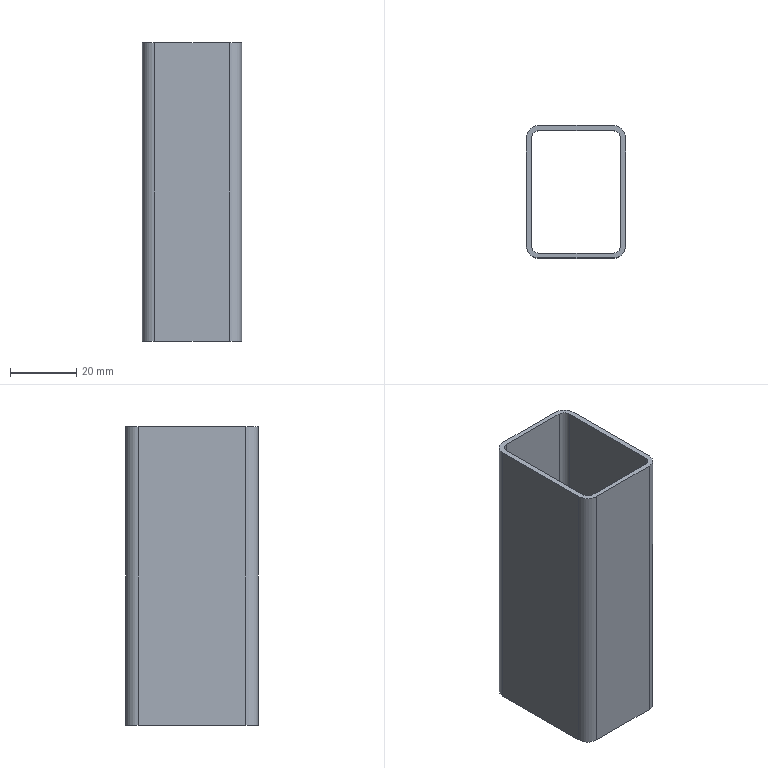Part | SolidWorks | features BaseBody 1 | 1 solid | 18 faces | box 30 x 40 x 90 mm | volume 17395 mm3 | plane 10 | cylinder 8 | commonest cylinder face diameters 4.5 x4 7.5 x4
STEP:
#1=CARTESIAN_POINT('',(11.25,18.5,90.));
#2=VERTEX_POINT('',#1);
#3=CARTESIAN_POINT('',(-11.25,18.5,90.));
#4=VERTEX_POINT('',#3);
#5=CARTESIAN_POINT('',(-5.625,18.5,90.));
#6=DIRECTION('',(-1.,0.,0.));
#7=VECTOR('',#6,1000.);
#8=LINE('',#5,#7);
#9=EDGE_CURVE('',#2,#4,#8,.T.);
#10=ORIENTED_EDGE('',*,*,#9,.F.);
#11=CARTESIAN_POINT('',(13.5,16.25,90.));
#12=VERTEX_POINT('',#11);
#13=CARTESIAN_POINT('',(11.25,16.25,90.));
#14=DIRECTION('',(0.,0.,1.));
#15=DIRECTION('',(-1.,0.,0.));
#16=AXIS2_PLACEMENT_3D('',#13,#14,#15);
#17=CIRCLE('',#16,2.25);
#18=EDGE_CURVE('',#12,#2,#17,.T.);
#19=ORIENTED_EDGE('',*,*,#18,.F.);
#20=CARTESIAN_POINT('',(13.5,-16.25,90.));
#21=VERTEX_POINT('',#20);
#22=CARTESIAN_POINT('',(13.5,8.125,90.));
#23=DIRECTION('',(0.,1.,0.));
#24=VECTOR('',#23,1000.);
#25=LINE('',#22,#24);
#26=EDGE_CURVE('',#21,#12,#25,.T.);
#27=ORIENTED_EDGE('',*,*,#26,.F.);
#28=CARTESIAN_POINT('',(11.25,-18.5,90.));
#29=VERTEX_POINT('',#28);
#30=CARTESIAN_POINT('',(11.25,-16.25,90.));
#31=DIRECTION('',(0.,0.,1.));
#32=DIRECTION('',(0.,1.,0.));
#33=AXIS2_PLACEMENT_3D('',#30,#31,#32);
#34=CIRCLE('',#33,2.25);
#35=EDGE_CURVE('',#29,#21,#34,.T.);
#36=ORIENTED_EDGE('',*,*,#35,.F.);
#37=CARTESIAN_POINT('',(-11.25,-18.5,90.));
#38=VERTEX_POINT('',#37);
#39=CARTESIAN_POINT('',(5.625,-18.5,90.));
#40=DIRECTION('',(1.,0.,0.));
#41=VECTOR('',#40,1000.);
#42=LINE('',#39,#41);
#43=EDGE_CURVE('',#38,#29,#42,.T.);
#44=ORIENTED_EDGE('',*,*,#43,.F.);
#45=CARTESIAN_POINT('',(-13.5,-16.25,90.));
#46=VERTEX_POINT('',#45);
#47=CARTESIAN_POINT('',(-11.25,-16.25,90.));
#48=DIRECTION('',(0.,0.,1.));
#49=DIRECTION('',(1.,0.,0.));
#50=AXIS2_PLACEMENT_3D('',#47,#48,#49);
#51=CIRCLE('',#50,2.25);
#52=EDGE_CURVE('',#46,#38,#51,.T.);
#53=ORIENTED_EDGE('',*,*,#52,.F.);
#54=CARTESIAN_POINT('',(-13.5,16.25,90.));
#55=VERTEX_POINT('',#54);
#56=CARTESIAN_POINT('',(-13.5,-8.125,90.));
#57=DIRECTION('',(0.,-1.,0.));
#58=VECTOR('',#57,1000.);
#59=LINE('',#56,#58);
#60=EDGE_CURVE('',#55,#46,#59,.T.);
#61=ORIENTED_EDGE('',*,*,#60,.F.);
#62=CARTESIAN_POINT('',(-11.25,16.25,90.));
#63=DIRECTION('',(0.,0.,1.));
#64=DIRECTION('',(0.,-1.,0.));
#65=AXIS2_PLACEMENT_3D('',#62,#63,#64);
#66=CIRCLE('',#65,2.25);
#67=EDGE_CURVE('',#4,#55,#66,.T.);
#68=ORIENTED_EDGE('',*,*,#67,.F.);
#69=EDGE_LOOP('',(#10,#19,#27,#36,#44,#53,#61,#68));
#70=FACE_BOUND('',#69,.T.);
#71=CARTESIAN_POINT('',(-15.,-16.25,90.));
#72=VERTEX_POINT('',#71);
#73=CARTESIAN_POINT('',(-15.,16.25,90.));
#74=VERTEX_POINT('',#73);
#75=CARTESIAN_POINT('',(-15.,-8.125,90.));
#76=DIRECTION('',(0.,1.,0.));
#77=VECTOR('',#76,1000.);
#78=LINE('',#75,#77);
#79=EDGE_CURVE('',#72,#74,#78,.T.);
#80=ORIENTED_EDGE('',*,*,#79,.F.);
#81=CARTESIAN_POINT('',(-11.25,-20.,90.));
#82=VERTEX_POINT('',#81);
#83=CARTESIAN_POINT('',(-11.25,-16.25,90.));
#84=DIRECTION('',(0.,0.,-1.));
#85=DIRECTION('',(1.,0.,0.));
#86=AXIS2_PLACEMENT_3D('',#83,#84,#85);
#87=CIRCLE('',#86,3.75);
#88=EDGE_CURVE('',#82,#72,#87,.T.);
#89=ORIENTED_EDGE('',*,*,#88,.F.);
#90=CARTESIAN_POINT('',(11.25,-20.,90.));
#91=VERTEX_POINT('',#90);
#92=CARTESIAN_POINT('',(5.625,-20.,90.));
#93=DIRECTION('',(-1.,0.,0.));
#94=VECTOR('',#93,1000.);
#95=LINE('',#92,#94);
#96=EDGE_CURVE('',#91,#82,#95,.T.);
#97=ORIENTED_EDGE('',*,*,#96,.F.);
#98=CARTESIAN_POINT('',(15.,-16.25,90.));
#99=VERTEX_POINT('',#98);
#100=CARTESIAN_POINT('',(11.25,-16.25,90.));
#101=DIRECTION('',(0.,0.,-1.));
#102=DIRECTION('',(0.,1.,0.));
#103=AXIS2_PLACEMENT_3D('',#100,#101,#102);
#104=CIRCLE('',#103,3.75);
#105=EDGE_CURVE('',#99,#91,#104,.T.);
#106=ORIENTED_EDGE('',*,*,#105,.F.);
#107=CARTESIAN_POINT('',(15.,16.25,90.));
#108=VERTEX_POINT('',#107);
#109=CARTESIAN_POINT('',(15.,8.125,90.));
#110=DIRECTION('',(0.,-1.,0.));
#111=VECTOR('',#110,1000.);
#112=LINE('',#109,#111);
#113=EDGE_CURVE('',#108,#99,#112,.T.);
#114=ORIENTED_EDGE('',*,*,#113,.F.);
#115=CARTESIAN_POINT('',(11.25,20.,90.));
#116=VERTEX_POINT('',#115);
#117=CARTESIAN_POINT('',(11.25,16.25,90.));
#118=DIRECTION('',(0.,0.,-1.));
#119=DIRECTION('',(-1.,0.,0.));
#120=AXIS2_PLACEMENT_3D('',#117,#118,#119);
#121=CIRCLE('',#120,3.75);
#122=EDGE_CURVE('',#116,#108,#121,.T.);
#123=ORIENTED_EDGE('',*,*,#122,.F.);
#124=CARTESIAN_POINT('',(-11.25,20.,90.));
#125=VERTEX_POINT('',#124);
#126=CARTESIAN_POINT('',(-5.625,20.,90.));
#127=DIRECTION('',(1.,0.,0.));
#128=VECTOR('',#127,1000.);
#129=LINE('',#126,#128);
#130=EDGE_CURVE('',#125,#116,#129,.T.);
#131=ORIENTED_EDGE('',*,*,#130,.F.);
#132=CARTESIAN_POINT('',(-11.25,16.25,90.));
#133=DIRECTION('',(0.,0.,-1.));
#134=DIRECTION('',(0.,-1.,0.));
#135=AXIS2_PLACEMENT_3D('',#132,#133,#134);
#136=CIRCLE('',#135,3.75);
#137=EDGE_CURVE('',#74,#125,#136,.T.);
#138=ORIENTED_EDGE('',*,*,#137,.F.);
#139=EDGE_LOOP('',(#80,#89,#97,#106,#114,#123,#131,#138));
#140=FACE_OUTER_BOUND('',#139,.T.);
#141=CARTESIAN_POINT('',(0.,0.,90.));
#142=DIRECTION('',(0.,0.,1.));
#143=DIRECTION('',(1.,0.,0.));
#144=AXIS2_PLACEMENT_3D('',#141,#142,#143);
#145=PLANE('',#144);
#146=ADVANCED_FACE('',(#70,#140),#145,.T.);
#147=CARTESIAN_POINT('',(11.25,18.5,0.));
#148=VERTEX_POINT('',#147);
#149=CARTESIAN_POINT('',(-11.25,18.5,0.));
#150=VERTEX_POINT('',#149);
#151=CARTESIAN_POINT('',(-5.625,18.5,0.));
#152=DIRECTION('',(-1.,0.,0.));
#153=VECTOR('',#152,1000.);
#154=LINE('',#151,#153);
#155=EDGE_CURVE('',#148,#150,#154,.T.);
#156=ORIENTED_EDGE('',*,*,#155,.T.);
#157=CARTESIAN_POINT('',(-13.5,16.25,0.));
#158=VERTEX_POINT('',#157);
#159=CARTESIAN_POINT('',(-11.25,16.25,0.));
#160=DIRECTION('',(0.,0.,1.));
#161=DIRECTION('',(0.,-1.,0.));
#162=AXIS2_PLACEMENT_3D('',#159,#160,#161);
#163=CIRCLE('',#162,2.25);
#164=EDGE_CURVE('',#150,#158,#163,.T.);
#165=ORIENTED_EDGE('',*,*,#164,.T.);
#166=CARTESIAN_POINT('',(-13.5,-16.25,0.));
#167=VERTEX_POINT('',#166);
#168=CARTESIAN_POINT('',(-13.5,-8.125,0.));
#169=DIRECTION('',(0.,-1.,0.));
#170=VECTOR('',#169,1000.);
#171=LINE('',#168,#170);
#172=EDGE_CURVE('',#158,#167,#171,.T.);
#173=ORIENTED_EDGE('',*,*,#172,.T.);
#174=CARTESIAN_POINT('',(-11.25,-18.5,0.));
#175=VERTEX_POINT('',#174);
#176=CARTESIAN_POINT('',(-11.25,-16.25,0.));
#177=DIRECTION('',(0.,0.,1.));
#178=DIRECTION('',(1.,0.,0.));
#179=AXIS2_PLACEMENT_3D('',#176,#177,#178);
#180=CIRCLE('',#179,2.25);
#181=EDGE_CURVE('',#167,#175,#180,.T.);
#182=ORIENTED_EDGE('',*,*,#181,.T.);
#183=CARTESIAN_POINT('',(11.25,-18.5,0.));
#184=VERTEX_POINT('',#183);
#185=CARTESIAN_POINT('',(5.625,-18.5,0.));
#186=DIRECTION('',(1.,0.,0.));
#187=VECTOR('',#186,1000.);
#188=LINE('',#185,#187);
#189=EDGE_CURVE('',#175,#184,#188,.T.);
#190=ORIENTED_EDGE('',*,*,#189,.T.);
#191=CARTESIAN_POINT('',(13.5,-16.25,0.));
#192=VERTEX_POINT('',#191);
#193=CARTESIAN_POINT('',(11.25,-16.25,0.));
#194=DIRECTION('',(0.,0.,1.));
#195=DIRECTION('',(0.,1.,0.));
#196=AXIS2_PLACEMENT_3D('',#193,#194,#195);
#197=CIRCLE('',#196,2.25);
#198=EDGE_CURVE('',#184,#192,#197,.T.);
#199=ORIENTED_EDGE('',*,*,#198,.T.);
#200=CARTESIAN_POINT('',(13.5,16.25,0.));
#201=VERTEX_POINT('',#200);
#202=CARTESIAN_POINT('',(13.5,8.125,0.));
#203=DIRECTION('',(0.,1.,0.));
#204=VECTOR('',#203,1000.);
#205=LINE('',#202,#204);
#206=EDGE_CURVE('',#192,#201,#205,.T.);
#207=ORIENTED_EDGE('',*,*,#206,.T.);
#208=CARTESIAN_POINT('',(11.25,16.25,0.));
#209=DIRECTION('',(0.,0.,1.));
#210=DIRECTION('',(-1.,0.,0.));
#211=AXIS2_PLACEMENT_3D('',#208,#209,#210);
#212=CIRCLE('',#211,2.25);
#213=EDGE_CURVE('',#201,#148,#212,.T.);
#214=ORIENTED_EDGE('',*,*,#213,.T.);
#215=EDGE_LOOP('',(#156,#165,#173,#182,#190,#199,#207,#214));
#216=FACE_BOUND('',#215,.T.);
#217=CARTESIAN_POINT('',(-15.,-16.25,0.));
#218=VERTEX_POINT('',#217);
#219=CARTESIAN_POINT('',(-15.,16.25,0.));
#220=VERTEX_POINT('',#219);
#221=CARTESIAN_POINT('',(-15.,-8.125,0.));
#222=DIRECTION('',(0.,1.,0.));
#223=VECTOR('',#222,1000.);
#224=LINE('',#221,#223);
#225=EDGE_CURVE('',#218,#220,#224,.T.);
#226=ORIENTED_EDGE('',*,*,#225,.T.);
#227=CARTESIAN_POINT('',(-11.25,20.,0.));
#228=VERTEX_POINT('',#227);
#229=CARTESIAN_POINT('',(-11.25,16.25,0.));
#230=DIRECTION('',(0.,0.,-1.));
#231=DIRECTION('',(0.,-1.,0.));
#232=AXIS2_PLACEMENT_3D('',#229,#230,#231);
#233=CIRCLE('',#232,3.75);
#234=EDGE_CURVE('',#220,#228,#233,.T.);
#235=ORIENTED_EDGE('',*,*,#234,.T.);
#236=CARTESIAN_POINT('',(11.25,20.,0.));
#237=VERTEX_POINT('',#236);
#238=CARTESIAN_POINT('',(-5.625,20.,0.));
#239=DIRECTION('',(1.,0.,0.));
#240=VECTOR('',#239,1000.);
#241=LINE('',#238,#240);
#242=EDGE_CURVE('',#228,#237,#241,.T.);
#243=ORIENTED_EDGE('',*,*,#242,.T.);
#244=CARTESIAN_POINT('',(15.,16.25,0.));
#245=VERTEX_POINT('',#244);
#246=CARTESIAN_POINT('',(11.25,16.25,0.));
#247=DIRECTION('',(0.,0.,-1.));
#248=DIRECTION('',(-1.,0.,0.));
#249=AXIS2_PLACEMENT_3D('',#246,#247,#248);
#250=CIRCLE('',#249,3.75);
#251=EDGE_CURVE('',#237,#245,#250,.T.);
#252=ORIENTED_EDGE('',*,*,#251,.T.);
#253=CARTESIAN_POINT('',(15.,-16.25,0.));
#254=VERTEX_POINT('',#253);
#255=CARTESIAN_POINT('',(15.,8.125,0.));
#256=DIRECTION('',(0.,-1.,0.));
#257=VECTOR('',#256,1000.);
#258=LINE('',#255,#257);
#259=EDGE_CURVE('',#245,#254,#258,.T.);
#260=ORIENTED_EDGE('',*,*,#259,.T.);
#261=CARTESIAN_POINT('',(11.25,-20.,0.));
#262=VERTEX_POINT('',#261);
#263=CARTESIAN_POINT('',(11.25,-16.25,0.));
#264=DIRECTION('',(0.,0.,-1.));
#265=DIRECTION('',(0.,1.,0.));
#266=AXIS2_PLACEMENT_3D('',#263,#264,#265);
#267=CIRCLE('',#266,3.75);
#268=EDGE_CURVE('',#254,#262,#267,.T.);
#269=ORIENTED_EDGE('',*,*,#268,.T.);
#270=CARTESIAN_POINT('',(-11.25,-20.,0.));
#271=VERTEX_POINT('',#270);
#272=CARTESIAN_POINT('',(5.625,-20.,0.));
#273=DIRECTION('',(-1.,0.,0.));
#274=VECTOR('',#273,1000.);
#275=LINE('',#272,#274);
#276=EDGE_CURVE('',#262,#271,#275,.T.);
#277=ORIENTED_EDGE('',*,*,#276,.T.);
#278=CARTESIAN_POINT('',(-11.25,-16.25,0.));
#279=DIRECTION('',(0.,0.,-1.));
#280=DIRECTION('',(1.,0.,0.));
#281=AXIS2_PLACEMENT_3D('',#278,#279,#280);
#282=CIRCLE('',#281,3.75);
#283=EDGE_CURVE('',#271,#218,#282,.T.);
#284=ORIENTED_EDGE('',*,*,#283,.T.);
#285=EDGE_LOOP('',(#226,#235,#243,#252,#260,#269,#277,#284));
#286=FACE_OUTER_BOUND('',#285,.T.);
#287=CARTESIAN_POINT('',(0.,0.,0.));
#288=DIRECTION('',(0.,0.,1.));
#289=DIRECTION('',(1.,0.,0.));
#290=AXIS2_PLACEMENT_3D('',#287,#288,#289);
#291=PLANE('',#290);
#292=ADVANCED_FACE('',(#216,#286),#291,.F.);
#293=ORIENTED_EDGE('',*,*,#122,.T.);
#294=CARTESIAN_POINT('',(15.,16.25,0.));
#295=DIRECTION('',(0.,0.,1.));
#296=VECTOR('',#295,1000.);
#297=LINE('',#294,#296);
#298=EDGE_CURVE('',#245,#108,#297,.T.);
#299=ORIENTED_EDGE('',*,*,#298,.F.);
#300=ORIENTED_EDGE('',*,*,#251,.F.);
#301=CARTESIAN_POINT('',(11.25,20.,0.));
#302=DIRECTION('',(0.,0.,1.));
#303=VECTOR('',#302,1000.);
#304=LINE('',#301,#303);
#305=EDGE_CURVE('',#237,#116,#304,.T.);
#306=ORIENTED_EDGE('',*,*,#305,.T.);
#307=EDGE_LOOP('',(#293,#299,#300,#306));
#308=FACE_OUTER_BOUND('',#307,.T.);
#309=CARTESIAN_POINT('',(11.25,16.25,0.));
#310=DIRECTION('',(0.,0.,1.));
#311=DIRECTION('',(-1.,0.,0.));
#312=AXIS2_PLACEMENT_3D('',#309,#310,#311);
#313=CYLINDRICAL_SURFACE('',#312,3.75);
#314=ADVANCED_FACE('',(#308),#313,.T.);
#315=ORIENTED_EDGE('',*,*,#130,.T.);
#316=ORIENTED_EDGE('',*,*,#305,.F.);
#317=ORIENTED_EDGE('',*,*,#242,.F.);
#318=CARTESIAN_POINT('',(-11.25,20.,0.));
#319=DIRECTION('',(0.,0.,1.));
#320=VECTOR('',#319,1000.);
#321=LINE('',#318,#320);
#322=EDGE_CURVE('',#228,#125,#321,.T.);
#323=ORIENTED_EDGE('',*,*,#322,.T.);
#324=EDGE_LOOP('',(#315,#316,#317,#323));
#325=FACE_OUTER_BOUND('',#324,.T.);
#326=CARTESIAN_POINT('',(-11.25,20.,0.));
#327=DIRECTION('',(0.,1.,0.));
#328=DIRECTION('',(1.,0.,0.));
#329=AXIS2_PLACEMENT_3D('',#326,#327,#328);
#330=PLANE('',#329);
#331=ADVANCED_FACE('',(#325),#330,.T.);
#332=ORIENTED_EDGE('',*,*,#137,.T.);
#333=ORIENTED_EDGE('',*,*,#322,.F.);
#334=ORIENTED_EDGE('',*,*,#234,.F.);
#335=CARTESIAN_POINT('',(-15.,16.25,0.));
#336=DIRECTION('',(0.,0.,1.));
#337=VECTOR('',#336,1000.);
#338=LINE('',#335,#337);
#339=EDGE_CURVE('',#220,#74,#338,.T.);
#340=ORIENTED_EDGE('',*,*,#339,.T.);
#341=EDGE_LOOP('',(#332,#333,#334,#340));
#342=FACE_OUTER_BOUND('',#341,.T.);
#343=CARTESIAN_POINT('',(-11.25,16.25,0.));
#344=DIRECTION('',(0.,0.,1.));
#345=DIRECTION('',(0.,-1.,0.));
#346=AXIS2_PLACEMENT_3D('',#343,#344,#345);
#347=CYLINDRICAL_SURFACE('',#346,3.75);
#348=ADVANCED_FACE('',(#342),#347,.T.);
#349=ORIENTED_EDGE('',*,*,#79,.T.);
#350=ORIENTED_EDGE('',*,*,#339,.F.);
#351=ORIENTED_EDGE('',*,*,#225,.F.);
#352=CARTESIAN_POINT('',(-15.,-16.25,0.));
#353=DIRECTION('',(0.,0.,1.));
#354=VECTOR('',#353,1000.);
#355=LINE('',#352,#354);
#356=EDGE_CURVE('',#218,#72,#355,.T.);
#357=ORIENTED_EDGE('',*,*,#356,.T.);
#358=EDGE_LOOP('',(#349,#350,#351,#357));
#359=FACE_OUTER_BOUND('',#358,.T.);
#360=CARTESIAN_POINT('',(-15.,-16.25,0.));
#361=DIRECTION('',(-1.,0.,0.));
#362=DIRECTION('',(0.,1.,0.));
#363=AXIS2_PLACEMENT_3D('',#360,#361,#362);
#364=PLANE('',#363);
#365=ADVANCED_FACE('',(#359),#364,.T.);
#366=ORIENTED_EDGE('',*,*,#67,.T.);
#367=CARTESIAN_POINT('',(-13.5,16.25,0.));
#368=DIRECTION('',(0.,0.,1.));
#369=VECTOR('',#368,1000.);
#370=LINE('',#367,#369);
#371=EDGE_CURVE('',#158,#55,#370,.T.);
#372=ORIENTED_EDGE('',*,*,#371,.F.);
#373=ORIENTED_EDGE('',*,*,#164,.F.);
#374=CARTESIAN_POINT('',(-11.25,18.5,0.));
#375=DIRECTION('',(0.,0.,1.));
#376=VECTOR('',#375,1000.);
#377=LINE('',#374,#376);
#378=EDGE_CURVE('',#150,#4,#377,.T.);
#379=ORIENTED_EDGE('',*,*,#378,.T.);
#380=EDGE_LOOP('',(#366,#372,#373,#379));
#381=FACE_OUTER_BOUND('',#380,.T.);
#382=CARTESIAN_POINT('',(-11.25,16.25,0.));
#383=DIRECTION('',(0.,0.,1.));
#384=DIRECTION('',(0.,-1.,0.));
#385=AXIS2_PLACEMENT_3D('',#382,#383,#384);
#386=CYLINDRICAL_SURFACE('',#385,2.25);
#387=ADVANCED_FACE('',(#381),#386,.F.);
#388=ORIENTED_EDGE('',*,*,#60,.T.);
#389=CARTESIAN_POINT('',(-13.5,-16.25,0.));
#390=DIRECTION('',(0.,0.,1.));
#391=VECTOR('',#390,1000.);
#392=LINE('',#389,#391);
#393=EDGE_CURVE('',#167,#46,#392,.T.);
#394=ORIENTED_EDGE('',*,*,#393,.F.);
#395=ORIENTED_EDGE('',*,*,#172,.F.);
#396=ORIENTED_EDGE('',*,*,#371,.T.);
#397=EDGE_LOOP('',(#388,#394,#395,#396));
#398=FACE_OUTER_BOUND('',#397,.T.);
#399=CARTESIAN_POINT('',(-13.5,-16.25,0.));
#400=DIRECTION('',(-1.,0.,0.));
#401=DIRECTION('',(0.,1.,0.));
#402=AXIS2_PLACEMENT_3D('',#399,#400,#401);
#403=PLANE('',#402);
#404=ADVANCED_FACE('',(#398),#403,.F.);
#405=ORIENTED_EDGE('',*,*,#52,.T.);
#406=CARTESIAN_POINT('',(-11.25,-18.5,0.));
#407=DIRECTION('',(0.,0.,1.));
#408=VECTOR('',#407,1000.);
#409=LINE('',#406,#408);
#410=EDGE_CURVE('',#175,#38,#409,.T.);
#411=ORIENTED_EDGE('',*,*,#410,.F.);
#412=ORIENTED_EDGE('',*,*,#181,.F.);
#413=ORIENTED_EDGE('',*,*,#393,.T.);
#414=EDGE_LOOP('',(#405,#411,#412,#413));
#415=FACE_OUTER_BOUND('',#414,.T.);
#416=CARTESIAN_POINT('',(-11.25,-16.25,0.));
#417=DIRECTION('',(0.,0.,1.));
#418=DIRECTION('',(1.,0.,0.));
#419=AXIS2_PLACEMENT_3D('',#416,#417,#418);
#420=CYLINDRICAL_SURFACE('',#419,2.25);
#421=ADVANCED_FACE('',(#415),#420,.F.);
#422=ORIENTED_EDGE('',*,*,#9,.T.);
#423=ORIENTED_EDGE('',*,*,#378,.F.);
#424=ORIENTED_EDGE('',*,*,#155,.F.);
#425=CARTESIAN_POINT('',(11.25,18.5,0.));
#426=DIRECTION('',(0.,0.,1.));
#427=VECTOR('',#426,1000.);
#428=LINE('',#425,#427);
#429=EDGE_CURVE('',#148,#2,#428,.T.);
#430=ORIENTED_EDGE('',*,*,#429,.T.);
#431=EDGE_LOOP('',(#422,#423,#424,#430));
#432=FACE_OUTER_BOUND('',#431,.T.);
#433=CARTESIAN_POINT('',(-11.25,18.5,0.));
#434=DIRECTION('',(0.,1.,0.));
#435=DIRECTION('',(1.,0.,0.));
#436=AXIS2_PLACEMENT_3D('',#433,#434,#435);
#437=PLANE('',#436);
#438=ADVANCED_FACE('',(#432),#437,.F.);
#439=ORIENTED_EDGE('',*,*,#88,.T.);
#440=ORIENTED_EDGE('',*,*,#356,.F.);
#441=ORIENTED_EDGE('',*,*,#283,.F.);
#442=CARTESIAN_POINT('',(-11.25,-20.,0.));
#443=DIRECTION('',(0.,0.,1.));
#444=VECTOR('',#443,1000.);
#445=LINE('',#442,#444);
#446=EDGE_CURVE('',#271,#82,#445,.T.);
#447=ORIENTED_EDGE('',*,*,#446,.T.);
#448=EDGE_LOOP('',(#439,#440,#441,#447));
#449=FACE_OUTER_BOUND('',#448,.T.);
#450=CARTESIAN_POINT('',(-11.25,-16.25,0.));
#451=DIRECTION('',(0.,0.,1.));
#452=DIRECTION('',(1.,0.,0.));
#453=AXIS2_PLACEMENT_3D('',#450,#451,#452);
#454=CYLINDRICAL_SURFACE('',#453,3.75);
#455=ADVANCED_FACE('',(#449),#454,.T.);
#456=ORIENTED_EDGE('',*,*,#96,.T.);
#457=ORIENTED_EDGE('',*,*,#446,.F.);
#458=ORIENTED_EDGE('',*,*,#276,.F.);
#459=CARTESIAN_POINT('',(11.25,-20.,0.));
#460=DIRECTION('',(0.,0.,1.));
#461=VECTOR('',#460,1000.);
#462=LINE('',#459,#461);
#463=EDGE_CURVE('',#262,#91,#462,.T.);
#464=ORIENTED_EDGE('',*,*,#463,.T.);
#465=EDGE_LOOP('',(#456,#457,#458,#464));
#466=FACE_OUTER_BOUND('',#465,.T.);
#467=CARTESIAN_POINT('',(11.25,-20.,0.));
#468=DIRECTION('',(0.,-1.,0.));
#469=DIRECTION('',(0.,0.,-1.));
#470=AXIS2_PLACEMENT_3D('',#467,#468,#469);
#471=PLANE('',#470);
#472=ADVANCED_FACE('',(#466),#471,.T.);
#473=ORIENTED_EDGE('',*,*,#105,.T.);
#474=ORIENTED_EDGE('',*,*,#463,.F.);
#475=ORIENTED_EDGE('',*,*,#268,.F.);
#476=CARTESIAN_POINT('',(15.,-16.25,0.));
#477=DIRECTION('',(0.,0.,1.));
#478=VECTOR('',#477,1000.);
#479=LINE('',#476,#478);
#480=EDGE_CURVE('',#254,#99,#479,.T.);
#481=ORIENTED_EDGE('',*,*,#480,.T.);
#482=EDGE_LOOP('',(#473,#474,#475,#481));
#483=FACE_OUTER_BOUND('',#482,.T.);
#484=CARTESIAN_POINT('',(11.25,-16.25,0.));
#485=DIRECTION('',(0.,0.,1.));
#486=DIRECTION('',(0.,1.,0.));
#487=AXIS2_PLACEMENT_3D('',#484,#485,#486);
#488=CYLINDRICAL_SURFACE('',#487,3.75);
#489=ADVANCED_FACE('',(#483),#488,.T.);
#490=ORIENTED_EDGE('',*,*,#113,.T.);
#491=ORIENTED_EDGE('',*,*,#480,.F.);
#492=ORIENTED_EDGE('',*,*,#259,.F.);
#493=ORIENTED_EDGE('',*,*,#298,.T.);
#494=EDGE_LOOP('',(#490,#491,#492,#493));
#495=FACE_OUTER_BOUND('',#494,.T.);
#496=CARTESIAN_POINT('',(15.,16.25,0.));
#497=DIRECTION('',(1.,0.,0.));
#498=DIRECTION('',(0.,1.,0.));
#499=AXIS2_PLACEMENT_3D('',#496,#497,#498);
#500=PLANE('',#499);
#501=ADVANCED_FACE('',(#495),#500,.T.);
#502=ORIENTED_EDGE('',*,*,#18,.T.);
#503=ORIENTED_EDGE('',*,*,#429,.F.);
#504=ORIENTED_EDGE('',*,*,#213,.F.);
#505=CARTESIAN_POINT('',(13.5,16.25,0.));
#506=DIRECTION('',(0.,0.,1.));
#507=VECTOR('',#506,1000.);
#508=LINE('',#505,#507);
#509=EDGE_CURVE('',#201,#12,#508,.T.);
#510=ORIENTED_EDGE('',*,*,#509,.T.);
#511=EDGE_LOOP('',(#502,#503,#504,#510));
#512=FACE_OUTER_BOUND('',#511,.T.);
#513=CARTESIAN_POINT('',(11.25,16.25,0.));
#514=DIRECTION('',(0.,0.,1.));
#515=DIRECTION('',(-1.,0.,0.));
#516=AXIS2_PLACEMENT_3D('',#513,#514,#515);
#517=CYLINDRICAL_SURFACE('',#516,2.25);
#518=ADVANCED_FACE('',(#512),#517,.F.);
#519=ORIENTED_EDGE('',*,*,#26,.T.);
#520=ORIENTED_EDGE('',*,*,#509,.F.);
#521=ORIENTED_EDGE('',*,*,#206,.F.);
#522=CARTESIAN_POINT('',(13.5,-16.25,0.));
#523=DIRECTION('',(0.,0.,1.));
#524=VECTOR('',#523,1000.);
#525=LINE('',#522,#524);
#526=EDGE_CURVE('',#192,#21,#525,.T.);
#527=ORIENTED_EDGE('',*,*,#526,.T.);
#528=EDGE_LOOP('',(#519,#520,#521,#527));
#529=FACE_OUTER_BOUND('',#528,.T.);
#530=CARTESIAN_POINT('',(13.5,16.25,0.));
#531=DIRECTION('',(1.,0.,0.));
#532=DIRECTION('',(0.,1.,0.));
#533=AXIS2_PLACEMENT_3D('',#530,#531,#532);
#534=PLANE('',#533);
#535=ADVANCED_FACE('',(#529),#534,.F.);
#536=ORIENTED_EDGE('',*,*,#35,.T.);
#537=ORIENTED_EDGE('',*,*,#526,.F.);
#538=ORIENTED_EDGE('',*,*,#198,.F.);
#539=CARTESIAN_POINT('',(11.25,-18.5,0.));
#540=DIRECTION('',(0.,0.,1.));
#541=VECTOR('',#540,1000.);
#542=LINE('',#539,#541);
#543=EDGE_CURVE('',#184,#29,#542,.T.);
#544=ORIENTED_EDGE('',*,*,#543,.T.);
#545=EDGE_LOOP('',(#536,#537,#538,#544));
#546=FACE_OUTER_BOUND('',#545,.T.);
#547=CARTESIAN_POINT('',(11.25,-16.25,0.));
#548=DIRECTION('',(0.,0.,1.));
#549=DIRECTION('',(0.,1.,0.));
#550=AXIS2_PLACEMENT_3D('',#547,#548,#549);
#551=CYLINDRICAL_SURFACE('',#550,2.25);
#552=ADVANCED_FACE('',(#546),#551,.F.);
#553=ORIENTED_EDGE('',*,*,#43,.T.);
#554=ORIENTED_EDGE('',*,*,#543,.F.);
#555=ORIENTED_EDGE('',*,*,#189,.F.);
#556=ORIENTED_EDGE('',*,*,#410,.T.);
#557=EDGE_LOOP('',(#553,#554,#555,#556));
#558=FACE_OUTER_BOUND('',#557,.T.);
#559=CARTESIAN_POINT('',(11.25,-18.5,0.));
#560=DIRECTION('',(0.,-1.,0.));
#561=DIRECTION('',(0.,0.,-1.));
#562=AXIS2_PLACEMENT_3D('',#559,#560,#561);
#563=PLANE('',#562);
#564=ADVANCED_FACE('',(#558),#563,.F.);
#565=CLOSED_SHELL('',(#146,#292,#314,#331,#348,#365,#387,#404,#421,#438,#455,#472,#489,#501,#518,#535,#552,#564));
#566=MANIFOLD_SOLID_BREP('',#565);
#567=CARTESIAN_POINT('',(0.,0.,0.));
#568=DIRECTION('',(0.,0.,1.));
#569=DIRECTION('',(1.,0.,0.));
#570=AXIS2_PLACEMENT_3D('',#567,#568,#569);
#571=(LENGTH_UNIT()NAMED_UNIT(*)SI_UNIT(.MILLI.,.METRE.));
#572=UNCERTAINTY_MEASURE_WITH_UNIT(LENGTH_MEASURE(0.00001),#571,'','');
#573=(NAMED_UNIT(*)PLANE_ANGLE_UNIT()SI_UNIT($,.RADIAN.));
#574=(NAMED_UNIT(*)SI_UNIT($,.STERADIAN.)SOLID_ANGLE_UNIT());
#575=(GEOMETRIC_REPRESENTATION_CONTEXT(3)GLOBAL_UNCERTAINTY_ASSIGNED_CONTEXT((#572))GLOBAL_UNIT_ASSIGNED_CONTEXT((#571,#573,#574))REPRESENTATION_CONTEXT('',''));
#576=ADVANCED_BREP_SHAPE_REPRESENTATION('',(#566,#570),#575);